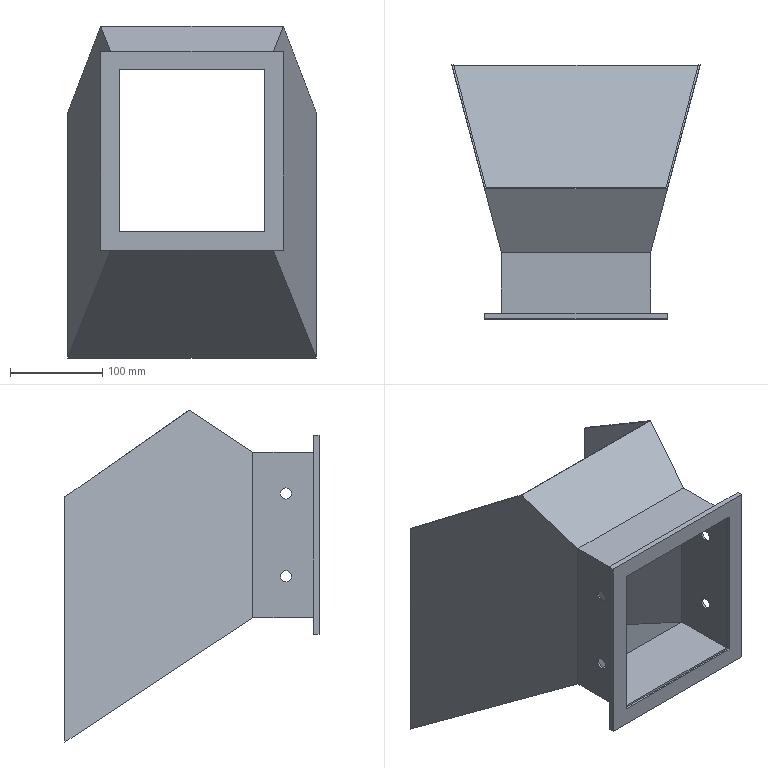Part | NX | 1 solid | 42 faces | box 270 x 276 x 360.692 mm | volume 479442 mm3 | plane 34 | cylinder 8 | commonest cylinder face diameters 12 x8
STEP:
#1=CARTESIAN_POINT('',(51.294,-541.499,2326.086));
#2=VERTEX_POINT('',#1);
#3=CARTESIAN_POINT('',(51.294,-541.499,2314.086));
#4=VERTEX_POINT('',#3);
#5=CARTESIAN_POINT('',(51.294,-541.499,2320.086));
#6=DIRECTION('',(1.,0.,0.));
#7=DIRECTION('',(0.,-1.,0.));
#8=AXIS2_PLACEMENT_3D('',#5,#6,#7);
#9=CIRCLE('',#8,6.);
#10=EDGE_CURVE('',#2,#4,#9,.T.);
#11=ORIENTED_EDGE('',*,*,#10,.T.);
#12=CARTESIAN_POINT('',(49.374,-541.499,2314.086));
#13=VERTEX_POINT('',#12);
#14=CARTESIAN_POINT('',(265.374,-541.499,2314.086));
#15=DIRECTION('',(1.,0.,0.));
#16=VECTOR('',#15,1.);
#17=LINE('',#14,#16);
#18=EDGE_CURVE('',#13,#4,#17,.T.);
#19=ORIENTED_EDGE('',*,*,#18,.F.);
#20=CARTESIAN_POINT('',(49.374,-541.499,2326.086));
#21=VERTEX_POINT('',#20);
#22=CARTESIAN_POINT('',(49.374,-541.499,2320.086));
#23=DIRECTION('',(1.,0.,0.));
#24=DIRECTION('',(0.,-1.,0.));
#25=AXIS2_PLACEMENT_3D('',#22,#23,#24);
#26=CIRCLE('',#25,6.);
#27=EDGE_CURVE('',#21,#13,#26,.T.);
#28=ORIENTED_EDGE('',*,*,#27,.F.);
#29=CARTESIAN_POINT('',(265.374,-541.499,2326.086));
#30=DIRECTION('',(-1.,0.,0.));
#31=VECTOR('',#30,1.);
#32=LINE('',#29,#31);
#33=EDGE_CURVE('',#2,#21,#32,.T.);
#34=ORIENTED_EDGE('',*,*,#33,.F.);
#35=EDGE_LOOP('',(#11,#19,#28,#34));
#36=FACE_OUTER_BOUND('',#35,.T.);
#37=CARTESIAN_POINT('',(265.374,-541.499,2320.086));
#38=DIRECTION('',(-1.,0.,0.));
#39=DIRECTION('',(0.,0.,1.));
#40=AXIS2_PLACEMENT_3D('',#37,#38,#39);
#41=CYLINDRICAL_SURFACE('',#40,6.);
#42=ADVANCED_FACE('',(#36),#41,.F.);
#43=CARTESIAN_POINT('',(211.374,-541.499,2314.086));
#44=VERTEX_POINT('',#43);
#45=CARTESIAN_POINT('',(211.374,-541.499,2326.086));
#46=VERTEX_POINT('',#45);
#47=CARTESIAN_POINT('',(211.374,-541.499,2320.086));
#48=DIRECTION('',(-1.,0.,0.));
#49=DIRECTION('',(0.,1.,0.));
#50=AXIS2_PLACEMENT_3D('',#47,#48,#49);
#51=CIRCLE('',#50,6.);
#52=EDGE_CURVE('',#44,#46,#51,.T.);
#53=ORIENTED_EDGE('',*,*,#52,.F.);
#54=CARTESIAN_POINT('',(209.454,-541.499,2314.086));
#55=VERTEX_POINT('',#54);
#56=CARTESIAN_POINT('',(265.374,-541.499,2314.086));
#57=DIRECTION('',(-1.,0.,0.));
#58=VECTOR('',#57,1.);
#59=LINE('',#56,#58);
#60=EDGE_CURVE('',#44,#55,#59,.T.);
#61=ORIENTED_EDGE('',*,*,#60,.T.);
#62=CARTESIAN_POINT('',(209.454,-541.499,2326.086));
#63=VERTEX_POINT('',#62);
#64=CARTESIAN_POINT('',(209.454,-541.499,2320.086));
#65=DIRECTION('',(-1.,0.,0.));
#66=DIRECTION('',(0.,1.,0.));
#67=AXIS2_PLACEMENT_3D('',#64,#65,#66);
#68=CIRCLE('',#67,6.);
#69=EDGE_CURVE('',#55,#63,#68,.T.);
#70=ORIENTED_EDGE('',*,*,#69,.T.);
#71=CARTESIAN_POINT('',(265.374,-541.499,2326.086));
#72=DIRECTION('',(1.,0.,0.));
#73=VECTOR('',#72,1.);
#74=LINE('',#71,#73);
#75=EDGE_CURVE('',#63,#46,#74,.T.);
#76=ORIENTED_EDGE('',*,*,#75,.T.);
#77=EDGE_LOOP('',(#53,#61,#70,#76));
#78=FACE_OUTER_BOUND('',#77,.T.);
#79=CARTESIAN_POINT('',(265.374,-541.499,2320.086));
#80=DIRECTION('',(-1.,0.,0.));
#81=DIRECTION('',(0.,0.,1.));
#82=AXIS2_PLACEMENT_3D('',#79,#80,#81);
#83=CYLINDRICAL_SURFACE('',#82,6.);
#84=ADVANCED_FACE('',(#78),#83,.F.);
#85=CARTESIAN_POINT('',(51.294,-541.499,2416.086));
#86=VERTEX_POINT('',#85);
#87=CARTESIAN_POINT('',(51.294,-541.499,2404.086));
#88=VERTEX_POINT('',#87);
#89=CARTESIAN_POINT('',(51.294,-541.499,2410.086));
#90=DIRECTION('',(1.,0.,0.));
#91=DIRECTION('',(0.,-1.,0.));
#92=AXIS2_PLACEMENT_3D('',#89,#90,#91);
#93=CIRCLE('',#92,6.);
#94=EDGE_CURVE('',#86,#88,#93,.T.);
#95=ORIENTED_EDGE('',*,*,#94,.T.);
#96=CARTESIAN_POINT('',(49.374,-541.499,2404.086));
#97=VERTEX_POINT('',#96);
#98=CARTESIAN_POINT('',(265.374,-541.499,2404.086));
#99=DIRECTION('',(1.,0.,0.));
#100=VECTOR('',#99,1.);
#101=LINE('',#98,#100);
#102=EDGE_CURVE('',#97,#88,#101,.T.);
#103=ORIENTED_EDGE('',*,*,#102,.F.);
#104=CARTESIAN_POINT('',(49.374,-541.499,2416.086));
#105=VERTEX_POINT('',#104);
#106=CARTESIAN_POINT('',(49.374,-541.499,2410.086));
#107=DIRECTION('',(1.,0.,0.));
#108=DIRECTION('',(0.,-1.,0.));
#109=AXIS2_PLACEMENT_3D('',#106,#107,#108);
#110=CIRCLE('',#109,6.);
#111=EDGE_CURVE('',#105,#97,#110,.T.);
#112=ORIENTED_EDGE('',*,*,#111,.F.);
#113=CARTESIAN_POINT('',(265.374,-541.499,2416.086));
#114=DIRECTION('',(-1.,0.,0.));
#115=VECTOR('',#114,1.);
#116=LINE('',#113,#115);
#117=EDGE_CURVE('',#86,#105,#116,.T.);
#118=ORIENTED_EDGE('',*,*,#117,.F.);
#119=EDGE_LOOP('',(#95,#103,#112,#118));
#120=FACE_OUTER_BOUND('',#119,.T.);
#121=CARTESIAN_POINT('',(265.374,-541.499,2410.086));
#122=DIRECTION('',(-1.,0.,0.));
#123=DIRECTION('',(0.,0.,1.));
#124=AXIS2_PLACEMENT_3D('',#121,#122,#123);
#125=CYLINDRICAL_SURFACE('',#124,6.);
#126=ADVANCED_FACE('',(#120),#125,.F.);
#127=CARTESIAN_POINT('',(211.374,-541.499,2404.086));
#128=VERTEX_POINT('',#127);
#129=CARTESIAN_POINT('',(211.374,-541.499,2416.086));
#130=VERTEX_POINT('',#129);
#131=CARTESIAN_POINT('',(211.374,-541.499,2410.086));
#132=DIRECTION('',(-1.,0.,0.));
#133=DIRECTION('',(0.,1.,0.));
#134=AXIS2_PLACEMENT_3D('',#131,#132,#133);
#135=CIRCLE('',#134,6.);
#136=EDGE_CURVE('',#128,#130,#135,.T.);
#137=ORIENTED_EDGE('',*,*,#136,.F.);
#138=CARTESIAN_POINT('',(209.454,-541.499,2404.086));
#139=VERTEX_POINT('',#138);
#140=CARTESIAN_POINT('',(265.374,-541.499,2404.086));
#141=DIRECTION('',(1.,0.,0.));
#142=VECTOR('',#141,1.);
#143=LINE('',#140,#142);
#144=EDGE_CURVE('',#139,#128,#143,.T.);
#145=ORIENTED_EDGE('',*,*,#144,.F.);
#146=CARTESIAN_POINT('',(209.454,-541.499,2416.086));
#147=VERTEX_POINT('',#146);
#148=CARTESIAN_POINT('',(209.454,-541.499,2410.086));
#149=DIRECTION('',(-1.,0.,0.));
#150=DIRECTION('',(0.,1.,0.));
#151=AXIS2_PLACEMENT_3D('',#148,#149,#150);
#152=CIRCLE('',#151,6.);
#153=EDGE_CURVE('',#139,#147,#152,.T.);
#154=ORIENTED_EDGE('',*,*,#153,.T.);
#155=CARTESIAN_POINT('',(265.374,-541.499,2416.086));
#156=DIRECTION('',(-1.,0.,0.));
#157=VECTOR('',#156,1.);
#158=LINE('',#155,#157);
#159=EDGE_CURVE('',#130,#147,#158,.T.);
#160=ORIENTED_EDGE('',*,*,#159,.F.);
#161=EDGE_LOOP('',(#137,#145,#154,#160));
#162=FACE_OUTER_BOUND('',#161,.T.);
#163=CARTESIAN_POINT('',(265.374,-541.499,2410.086));
#164=DIRECTION('',(-1.,0.,0.));
#165=DIRECTION('',(0.,0.,1.));
#166=AXIS2_PLACEMENT_3D('',#163,#164,#165);
#167=CYLINDRICAL_SURFACE('',#166,6.);
#168=ADVANCED_FACE('',(#162),#167,.F.);
#169=CARTESIAN_POINT('',(-4.626,-301.499,2140.086));
#170=VERTEX_POINT('',#169);
#171=CARTESIAN_POINT('',(-4.626,-301.499,2406.357));
#172=VERTEX_POINT('',#171);
#173=CARTESIAN_POINT('',(-4.626,-301.499,2590.086));
#174=DIRECTION('',(0.,0.,1.));
#175=VECTOR('',#174,1.);
#176=LINE('',#173,#175);
#177=EDGE_CURVE('',#170,#172,#176,.T.);
#178=ORIENTED_EDGE('',*,*,#177,.T.);
#179=CARTESIAN_POINT('',(-2.64,-301.499,2406.357));
#180=VERTEX_POINT('',#179);
#181=CARTESIAN_POINT('',(265.374,-301.499,2406.357));
#182=DIRECTION('',(1.,0.,0.));
#183=VECTOR('',#182,1.);
#184=LINE('',#181,#183);
#185=EDGE_CURVE('',#172,#180,#184,.T.);
#186=ORIENTED_EDGE('',*,*,#185,.T.);
#187=CARTESIAN_POINT('',(-2.64,-301.499,2142.389));
#188=VERTEX_POINT('',#187);
#189=CARTESIAN_POINT('',(-2.64,-301.499,2590.086));
#190=DIRECTION('',(0.,0.,1.));
#191=VECTOR('',#190,1.);
#192=LINE('',#189,#191);
#193=EDGE_CURVE('',#188,#180,#192,.T.);
#194=ORIENTED_EDGE('',*,*,#193,.F.);
#195=CARTESIAN_POINT('',(263.387,-301.499,2142.389));
#196=VERTEX_POINT('',#195);
#197=CARTESIAN_POINT('',(265.374,-301.499,2142.389));
#198=DIRECTION('',(-1.,0.,0.));
#199=VECTOR('',#198,1.);
#200=LINE('',#197,#199);
#201=EDGE_CURVE('',#196,#188,#200,.T.);
#202=ORIENTED_EDGE('',*,*,#201,.F.);
#203=CARTESIAN_POINT('',(263.387,-301.499,2406.357));
#204=VERTEX_POINT('',#203);
#205=CARTESIAN_POINT('',(263.387,-301.499,2140.086));
#206=DIRECTION('',(0.,0.,1.));
#207=VECTOR('',#206,1.);
#208=LINE('',#205,#207);
#209=EDGE_CURVE('',#196,#204,#208,.T.);
#210=ORIENTED_EDGE('',*,*,#209,.T.);
#211=CARTESIAN_POINT('',(265.374,-301.499,2406.357));
#212=VERTEX_POINT('',#211);
#213=CARTESIAN_POINT('',(265.374,-301.499,2406.357));
#214=DIRECTION('',(1.,0.,0.));
#215=VECTOR('',#214,1.);
#216=LINE('',#213,#215);
#217=EDGE_CURVE('',#204,#212,#216,.T.);
#218=ORIENTED_EDGE('',*,*,#217,.T.);
#219=CARTESIAN_POINT('',(265.374,-301.499,2140.086));
#220=VERTEX_POINT('',#219);
#221=CARTESIAN_POINT('',(265.374,-301.499,2590.086));
#222=DIRECTION('',(0.,0.,1.));
#223=VECTOR('',#222,1.);
#224=LINE('',#221,#223);
#225=EDGE_CURVE('',#220,#212,#224,.T.);
#226=ORIENTED_EDGE('',*,*,#225,.F.);
#227=CARTESIAN_POINT('',(265.374,-301.499,2140.086));
#228=DIRECTION('',(-1.,0.,0.));
#229=VECTOR('',#228,1.);
#230=LINE('',#227,#229);
#231=EDGE_CURVE('',#220,#170,#230,.T.);
#232=ORIENTED_EDGE('',*,*,#231,.T.);
#233=EDGE_LOOP('',(#178,#186,#194,#202,#210,#218,#226,#232));
#234=FACE_OUTER_BOUND('',#233,.T.);
#235=CARTESIAN_POINT('',(265.374,-301.499,2590.086));
#236=DIRECTION('',(0.,-1.,0.));
#237=DIRECTION('',(0.,0.,-1.));
#238=AXIS2_PLACEMENT_3D('',#235,#236,#237);
#239=PLANE('',#238);
#240=ADVANCED_FACE('',(#234),#239,.F.);
#241=CARTESIAN_POINT('',(211.374,-571.499,2455.086));
#242=VERTEX_POINT('',#241);
#243=CARTESIAN_POINT('',(49.374,-571.499,2455.086));
#244=VERTEX_POINT('',#243);
#245=CARTESIAN_POINT('',(265.374,-571.499,2455.086));
#246=DIRECTION('',(-1.,0.,0.));
#247=VECTOR('',#246,1.);
#248=LINE('',#245,#247);
#249=EDGE_CURVE('',#242,#244,#248,.T.);
#250=ORIENTED_EDGE('',*,*,#249,.F.);
#251=CARTESIAN_POINT('',(211.374,-505.499,2455.086));
#252=VERTEX_POINT('',#251);
#253=CARTESIAN_POINT('',(211.374,-571.499,2455.086));
#254=DIRECTION('',(0.,1.,0.));
#255=VECTOR('',#254,1.);
#256=LINE('',#253,#255);
#257=EDGE_CURVE('',#242,#252,#256,.T.);
#258=ORIENTED_EDGE('',*,*,#257,.T.);
#259=CARTESIAN_POINT('',(49.374,-505.499,2455.086));
#260=VERTEX_POINT('',#259);
#261=CARTESIAN_POINT('',(265.374,-505.499,2455.086));
#262=DIRECTION('',(-1.,0.,0.));
#263=VECTOR('',#262,1.);
#264=LINE('',#261,#263);
#265=EDGE_CURVE('',#252,#260,#264,.T.);
#266=ORIENTED_EDGE('',*,*,#265,.T.);
#267=CARTESIAN_POINT('',(49.374,-571.499,2455.086));
#268=DIRECTION('',(0.,-1.,0.));
#269=VECTOR('',#268,1.);
#270=LINE('',#267,#269);
#271=EDGE_CURVE('',#260,#244,#270,.T.);
#272=ORIENTED_EDGE('',*,*,#271,.T.);
#273=EDGE_LOOP('',(#250,#258,#266,#272));
#274=FACE_OUTER_BOUND('',#273,.T.);
#275=CARTESIAN_POINT('',(265.374,-571.499,2455.086));
#276=DIRECTION('',(0.,0.,-1.));
#277=DIRECTION('',(-1.,0.,0.));
#278=AXIS2_PLACEMENT_3D('',#275,#276,#277);
#279=PLANE('',#278);
#280=ADVANCED_FACE('',(#274),#279,.F.);
#281=CARTESIAN_POINT('',(211.374,-505.499,2275.086));
#282=VERTEX_POINT('',#281);
#283=CARTESIAN_POINT('',(49.374,-505.499,2275.086));
#284=VERTEX_POINT('',#283);
#285=CARTESIAN_POINT('',(265.374,-505.499,2275.086));
#286=DIRECTION('',(-1.,0.,0.));
#287=VECTOR('',#286,1.);
#288=LINE('',#285,#287);
#289=EDGE_CURVE('',#282,#284,#288,.T.);
#290=ORIENTED_EDGE('',*,*,#289,.F.);
#291=CARTESIAN_POINT('',(211.374,-571.499,2275.086));
#292=VERTEX_POINT('',#291);
#293=CARTESIAN_POINT('',(211.374,-571.499,2275.086));
#294=DIRECTION('',(0.,-1.,0.));
#295=VECTOR('',#294,1.);
#296=LINE('',#293,#295);
#297=EDGE_CURVE('',#282,#292,#296,.T.);
#298=ORIENTED_EDGE('',*,*,#297,.T.);
#299=CARTESIAN_POINT('',(49.374,-571.499,2275.086));
#300=VERTEX_POINT('',#299);
#301=CARTESIAN_POINT('',(265.374,-571.499,2275.086));
#302=DIRECTION('',(-1.,0.,0.));
#303=VECTOR('',#302,1.);
#304=LINE('',#301,#303);
#305=EDGE_CURVE('',#292,#300,#304,.T.);
#306=ORIENTED_EDGE('',*,*,#305,.T.);
#307=CARTESIAN_POINT('',(49.374,-571.499,2275.086));
#308=DIRECTION('',(0.,1.,0.));
#309=VECTOR('',#308,1.);
#310=LINE('',#307,#309);
#311=EDGE_CURVE('',#300,#284,#310,.T.);
#312=ORIENTED_EDGE('',*,*,#311,.T.);
#313=EDGE_LOOP('',(#290,#298,#306,#312));
#314=FACE_OUTER_BOUND('',#313,.T.);
#315=CARTESIAN_POINT('',(265.374,-571.499,2275.086));
#316=DIRECTION('',(0.,0.,1.));
#317=DIRECTION('',(0.,-1.,0.));
#318=AXIS2_PLACEMENT_3D('',#315,#316,#317);
#319=PLANE('',#318);
#320=ADVANCED_FACE('',(#314),#319,.F.);
#321=ORIENTED_EDGE('',*,*,#231,.F.);
#322=CARTESIAN_POINT('',(265.374,-301.499,2140.086));
#323=DIRECTION('',(-0.2156,-0.8143,0.5389));
#324=VECTOR('',#323,1.);
#325=LINE('',#322,#324);
#326=EDGE_CURVE('',#220,#282,#325,.T.);
#327=ORIENTED_EDGE('',*,*,#326,.T.);
#328=ORIENTED_EDGE('',*,*,#289,.T.);
#329=CARTESIAN_POINT('',(7.919,-348.894,2171.45));
#330=DIRECTION('',(-0.2156,0.8143,-0.5389));
#331=VECTOR('',#330,1.);
#332=LINE('',#329,#331);
#333=EDGE_CURVE('',#284,#170,#332,.T.);
#334=ORIENTED_EDGE('',*,*,#333,.T.);
#335=EDGE_LOOP('',(#321,#327,#328,#334));
#336=FACE_OUTER_BOUND('',#335,.T.);
#337=CARTESIAN_POINT('',(265.374,-301.499,2140.086));
#338=DIRECTION('',(0.,0.5519,0.8339));
#339=DIRECTION('',(0.,-0.8339,0.5519));
#340=AXIS2_PLACEMENT_3D('',#337,#338,#339);
#341=PLANE('',#340);
#342=ADVANCED_FACE('',(#336),#341,.F.);
#343=CARTESIAN_POINT('',(229.65,-436.453,2500.778));
#344=VERTEX_POINT('',#343);
#345=CARTESIAN_POINT('',(265.374,-301.499,2590.086));
#346=DIRECTION('',(0.2156,0.8143,0.5389));
#347=VECTOR('',#346,1.);
#348=LINE('',#345,#347);
#349=EDGE_CURVE('',#252,#344,#348,.T.);
#350=ORIENTED_EDGE('',*,*,#349,.T.);
#351=CARTESIAN_POINT('',(31.097,-436.453,2500.778));
#352=VERTEX_POINT('',#351);
#353=CARTESIAN_POINT('',(265.374,-436.453,2500.778));
#354=DIRECTION('',(-1.,0.,0.));
#355=VECTOR('',#354,1.);
#356=LINE('',#353,#355);
#357=EDGE_CURVE('',#344,#352,#356,.T.);
#358=ORIENTED_EDGE('',*,*,#357,.T.);
#359=CARTESIAN_POINT('',(7.919,-348.894,2558.722));
#360=DIRECTION('',(0.2156,-0.8143,-0.5389));
#361=VECTOR('',#360,1.);
#362=LINE('',#359,#361);
#363=EDGE_CURVE('',#352,#260,#362,.T.);
#364=ORIENTED_EDGE('',*,*,#363,.T.);
#365=ORIENTED_EDGE('',*,*,#265,.F.);
#366=EDGE_LOOP('',(#350,#358,#364,#365));
#367=FACE_OUTER_BOUND('',#366,.T.);
#368=CARTESIAN_POINT('',(265.374,-301.499,2590.086));
#369=DIRECTION('',(0.,0.5519,-0.8339));
#370=DIRECTION('',(0.,0.8339,0.5519));
#371=AXIS2_PLACEMENT_3D('',#368,#369,#370);
#372=PLANE('',#371);
#373=ADVANCED_FACE('',(#367),#372,.F.);
#374=ORIENTED_EDGE('',*,*,#27,.T.);
#375=CARTESIAN_POINT('',(49.374,-541.499,2320.086));
#376=DIRECTION('',(1.,0.,0.));
#377=DIRECTION('',(0.,-1.,0.));
#378=AXIS2_PLACEMENT_3D('',#375,#376,#377);
#379=CIRCLE('',#378,6.);
#380=EDGE_CURVE('',#13,#21,#379,.T.);
#381=ORIENTED_EDGE('',*,*,#380,.T.);
#382=EDGE_LOOP('',(#374,#381));
#383=FACE_BOUND('',#382,.T.);
#384=ORIENTED_EDGE('',*,*,#111,.T.);
#385=CARTESIAN_POINT('',(49.374,-541.499,2410.086));
#386=DIRECTION('',(1.,0.,0.));
#387=DIRECTION('',(0.,-1.,0.));
#388=AXIS2_PLACEMENT_3D('',#385,#386,#387);
#389=CIRCLE('',#388,6.);
#390=EDGE_CURVE('',#97,#105,#389,.T.);
#391=ORIENTED_EDGE('',*,*,#390,.T.);
#392=EDGE_LOOP('',(#384,#391));
#393=FACE_BOUND('',#392,.T.);
#394=CARTESIAN_POINT('',(49.374,-505.499,2140.086));
#395=DIRECTION('',(0.,0.,1.));
#396=VECTOR('',#395,1.);
#397=LINE('',#394,#396);
#398=EDGE_CURVE('',#284,#260,#397,.T.);
#399=ORIENTED_EDGE('',*,*,#398,.F.);
#400=ORIENTED_EDGE('',*,*,#311,.F.);
#401=CARTESIAN_POINT('',(49.374,-571.499,2140.086));
#402=DIRECTION('',(0.,0.,1.));
#403=VECTOR('',#402,1.);
#404=LINE('',#401,#403);
#405=EDGE_CURVE('',#300,#244,#404,.T.);
#406=ORIENTED_EDGE('',*,*,#405,.T.);
#407=ORIENTED_EDGE('',*,*,#271,.F.);
#408=EDGE_LOOP('',(#399,#400,#406,#407));
#409=FACE_BOUND('',#408,.T.);
#410=CARTESIAN_POINT('',(49.374,-505.499,2140.086));
#411=DIRECTION('',(1.,0.,0.));
#412=DIRECTION('',(0.,-1.,0.));
#413=AXIS2_PLACEMENT_3D('',#410,#411,#412);
#414=PLANE('',#413);
#415=ADVANCED_FACE('',(#383,#393,#409),#414,.F.);
#416=ORIENTED_EDGE('',*,*,#363,.F.);
#417=CARTESIAN_POINT('',(-36.246,-182.046,2322.78));
#418=DIRECTION('',(-0.212,0.8007,-0.5602));
#419=VECTOR('',#418,1.);
#420=LINE('',#417,#419);
#421=EDGE_CURVE('',#352,#172,#420,.T.);
#422=ORIENTED_EDGE('',*,*,#421,.T.);
#423=ORIENTED_EDGE('',*,*,#177,.F.);
#424=ORIENTED_EDGE('',*,*,#333,.F.);
#425=ORIENTED_EDGE('',*,*,#398,.T.);
#426=EDGE_LOOP('',(#416,#422,#423,#424,#425));
#427=FACE_OUTER_BOUND('',#426,.T.);
#428=CARTESIAN_POINT('',(-4.626,-301.499,2140.086));
#429=DIRECTION('',(0.9667,0.2559,0.));
#430=DIRECTION('',(0.2559,-0.9667,0.));
#431=AXIS2_PLACEMENT_3D('',#428,#429,#430);
#432=PLANE('',#431);
#433=ADVANCED_FACE('',(#427),#432,.F.);
#434=CARTESIAN_POINT('',(211.374,-541.499,2320.086));
#435=DIRECTION('',(-1.,0.,0.));
#436=DIRECTION('',(0.,1.,0.));
#437=AXIS2_PLACEMENT_3D('',#434,#435,#436);
#438=CIRCLE('',#437,6.);
#439=EDGE_CURVE('',#46,#44,#438,.T.);
#440=ORIENTED_EDGE('',*,*,#439,.T.);
#441=ORIENTED_EDGE('',*,*,#52,.T.);
#442=EDGE_LOOP('',(#440,#441));
#443=FACE_BOUND('',#442,.T.);
#444=CARTESIAN_POINT('',(211.374,-541.499,2410.086));
#445=DIRECTION('',(-1.,0.,0.));
#446=DIRECTION('',(0.,1.,0.));
#447=AXIS2_PLACEMENT_3D('',#444,#445,#446);
#448=CIRCLE('',#447,6.);
#449=EDGE_CURVE('',#130,#128,#448,.T.);
#450=ORIENTED_EDGE('',*,*,#449,.T.);
#451=ORIENTED_EDGE('',*,*,#136,.T.);
#452=EDGE_LOOP('',(#450,#451));
#453=FACE_BOUND('',#452,.T.);
#454=CARTESIAN_POINT('',(211.374,-571.499,2140.086));
#455=DIRECTION('',(0.,0.,1.));
#456=VECTOR('',#455,1.);
#457=LINE('',#454,#456);
#458=EDGE_CURVE('',#292,#242,#457,.T.);
#459=ORIENTED_EDGE('',*,*,#458,.F.);
#460=ORIENTED_EDGE('',*,*,#297,.F.);
#461=CARTESIAN_POINT('',(211.374,-505.499,2140.086));
#462=DIRECTION('',(0.,0.,1.));
#463=VECTOR('',#462,1.);
#464=LINE('',#461,#463);
#465=EDGE_CURVE('',#282,#252,#464,.T.);
#466=ORIENTED_EDGE('',*,*,#465,.T.);
#467=ORIENTED_EDGE('',*,*,#257,.F.);
#468=EDGE_LOOP('',(#459,#460,#466,#467));
#469=FACE_BOUND('',#468,.T.);
#470=CARTESIAN_POINT('',(211.374,-505.499,2140.086));
#471=DIRECTION('',(-1.,0.,0.));
#472=DIRECTION('',(0.,1.,0.));
#473=AXIS2_PLACEMENT_3D('',#470,#471,#472);
#474=PLANE('',#473);
#475=ADVANCED_FACE('',(#443,#453,#469),#474,.F.);
#476=ORIENTED_EDGE('',*,*,#225,.T.);
#477=CARTESIAN_POINT('',(296.994,-182.046,2322.78));
#478=DIRECTION('',(-0.212,-0.8007,0.5602));
#479=VECTOR('',#478,1.);
#480=LINE('',#477,#479);
#481=EDGE_CURVE('',#212,#344,#480,.T.);
#482=ORIENTED_EDGE('',*,*,#481,.T.);
#483=ORIENTED_EDGE('',*,*,#349,.F.);
#484=ORIENTED_EDGE('',*,*,#465,.F.);
#485=ORIENTED_EDGE('',*,*,#326,.F.);
#486=EDGE_LOOP('',(#476,#482,#483,#484,#485));
#487=FACE_OUTER_BOUND('',#486,.T.);
#488=CARTESIAN_POINT('',(265.374,-301.499,2140.086));
#489=DIRECTION('',(-0.9667,0.2559,0.));
#490=DIRECTION('',(0.2559,0.9667,0.));
#491=AXIS2_PLACEMENT_3D('',#488,#489,#490);
#492=PLANE('',#491);
#493=ADVANCED_FACE('',(#487),#492,.F.);
#494=CARTESIAN_POINT('',(229.374,-571.499,2473.086));
#495=VERTEX_POINT('',#494);
#496=CARTESIAN_POINT('',(31.374,-571.499,2473.086));
#497=VERTEX_POINT('',#496);
#498=CARTESIAN_POINT('',(229.374,-571.499,2473.086));
#499=DIRECTION('',(-1.,0.,0.));
#500=VECTOR('',#499,1.);
#501=LINE('',#498,#500);
#502=EDGE_CURVE('',#495,#497,#501,.T.);
#503=ORIENTED_EDGE('',*,*,#502,.F.);
#504=CARTESIAN_POINT('',(229.374,-571.499,2257.086));
#505=VERTEX_POINT('',#504);
#506=CARTESIAN_POINT('',(229.374,-571.499,2257.086));
#507=DIRECTION('',(0.,0.,1.));
#508=VECTOR('',#507,1.);
#509=LINE('',#506,#508);
#510=EDGE_CURVE('',#505,#495,#509,.T.);
#511=ORIENTED_EDGE('',*,*,#510,.F.);
#512=CARTESIAN_POINT('',(31.374,-571.499,2257.086));
#513=VERTEX_POINT('',#512);
#514=CARTESIAN_POINT('',(31.374,-571.499,2257.086));
#515=DIRECTION('',(1.,0.,0.));
#516=VECTOR('',#515,1.);
#517=LINE('',#514,#516);
#518=EDGE_CURVE('',#513,#505,#517,.T.);
#519=ORIENTED_EDGE('',*,*,#518,.F.);
#520=CARTESIAN_POINT('',(31.374,-571.499,2473.086));
#521=DIRECTION('',(0.,0.,-1.));
#522=VECTOR('',#521,1.);
#523=LINE('',#520,#522);
#524=EDGE_CURVE('',#497,#513,#523,.T.);
#525=ORIENTED_EDGE('',*,*,#524,.F.);
#526=EDGE_LOOP('',(#503,#511,#519,#525));
#527=FACE_BOUND('',#526,.T.);
#528=ORIENTED_EDGE('',*,*,#249,.T.);
#529=ORIENTED_EDGE('',*,*,#405,.F.);
#530=ORIENTED_EDGE('',*,*,#305,.F.);
#531=ORIENTED_EDGE('',*,*,#458,.T.);
#532=EDGE_LOOP('',(#528,#529,#530,#531));
#533=FACE_BOUND('',#532,.T.);
#534=CARTESIAN_POINT('',(31.374,-571.499,2473.086));
#535=DIRECTION('',(0.,-1.,0.));
#536=DIRECTION('',(-1.,0.,0.));
#537=AXIS2_PLACEMENT_3D('',#534,#535,#536);
#538=PLANE('',#537);
#539=ADVANCED_FACE('',(#527,#533),#538,.F.);
#540=ORIENTED_EDGE('',*,*,#502,.T.);
#541=CARTESIAN_POINT('',(31.374,-577.499,2473.086));
#542=VERTEX_POINT('',#541);
#543=CARTESIAN_POINT('',(31.374,-577.499,2473.086));
#544=DIRECTION('',(0.,1.,0.));
#545=VECTOR('',#544,1.);
#546=LINE('',#543,#545);
#547=EDGE_CURVE('',#542,#497,#546,.T.);
#548=ORIENTED_EDGE('',*,*,#547,.F.);
#549=CARTESIAN_POINT('',(229.374,-577.499,2473.086));
#550=VERTEX_POINT('',#549);
#551=CARTESIAN_POINT('',(229.374,-577.499,2473.086));
#552=DIRECTION('',(-1.,0.,0.));
#553=VECTOR('',#552,1.);
#554=LINE('',#551,#553);
#555=EDGE_CURVE('',#550,#542,#554,.T.);
#556=ORIENTED_EDGE('',*,*,#555,.F.);
#557=CARTESIAN_POINT('',(229.374,-577.499,2473.086));
#558=DIRECTION('',(0.,1.,0.));
#559=VECTOR('',#558,1.);
#560=LINE('',#557,#559);
#561=EDGE_CURVE('',#550,#495,#560,.T.);
#562=ORIENTED_EDGE('',*,*,#561,.T.);
#563=EDGE_LOOP('',(#540,#548,#556,#562));
#564=FACE_OUTER_BOUND('',#563,.T.);
#565=CARTESIAN_POINT('',(229.374,-577.499,2473.086));
#566=DIRECTION('',(0.,0.,-1.));
#567=DIRECTION('',(-1.,0.,0.));
#568=AXIS2_PLACEMENT_3D('',#565,#566,#567);
#569=PLANE('',#568);
#570=ADVANCED_FACE('',(#564),#569,.F.);
#571=ORIENTED_EDGE('',*,*,#524,.T.);
#572=CARTESIAN_POINT('',(31.374,-577.499,2257.086));
#573=VERTEX_POINT('',#572);
#574=CARTESIAN_POINT('',(31.374,-577.499,2257.086));
#575=DIRECTION('',(0.,1.,0.));
#576=VECTOR('',#575,1.);
#577=LINE('',#574,#576);
#578=EDGE_CURVE('',#573,#513,#577,.T.);
#579=ORIENTED_EDGE('',*,*,#578,.F.);
#580=CARTESIAN_POINT('',(31.374,-577.499,2473.086));
#581=DIRECTION('',(0.,0.,-1.));
#582=VECTOR('',#581,1.);
#583=LINE('',#580,#582);
#584=EDGE_CURVE('',#542,#573,#583,.T.);
#585=ORIENTED_EDGE('',*,*,#584,.F.);
#586=ORIENTED_EDGE('',*,*,#547,.T.);
#587=EDGE_LOOP('',(#571,#579,#585,#586));
#588=FACE_OUTER_BOUND('',#587,.T.);
#589=CARTESIAN_POINT('',(31.374,-577.499,2473.086));
#590=DIRECTION('',(1.,0.,0.));
#591=DIRECTION('',(0.,0.,-1.));
#592=AXIS2_PLACEMENT_3D('',#589,#590,#591);
#593=PLANE('',#592);
#594=ADVANCED_FACE('',(#588),#593,.F.);
#595=ORIENTED_EDGE('',*,*,#518,.T.);
#596=CARTESIAN_POINT('',(229.374,-577.499,2257.086));
#597=VERTEX_POINT('',#596);
#598=CARTESIAN_POINT('',(229.374,-577.499,2257.086));
#599=DIRECTION('',(0.,1.,0.));
#600=VECTOR('',#599,1.);
#601=LINE('',#598,#600);
#602=EDGE_CURVE('',#597,#505,#601,.T.);
#603=ORIENTED_EDGE('',*,*,#602,.F.);
#604=CARTESIAN_POINT('',(31.374,-577.499,2257.086));
#605=DIRECTION('',(1.,0.,0.));
#606=VECTOR('',#605,1.);
#607=LINE('',#604,#606);
#608=EDGE_CURVE('',#573,#597,#607,.T.);
#609=ORIENTED_EDGE('',*,*,#608,.F.);
#610=ORIENTED_EDGE('',*,*,#578,.T.);
#611=EDGE_LOOP('',(#595,#603,#609,#610));
#612=FACE_OUTER_BOUND('',#611,.T.);
#613=CARTESIAN_POINT('',(31.374,-577.499,2257.086));
#614=DIRECTION('',(0.,0.,1.));
#615=DIRECTION('',(1.,0.,0.));
#616=AXIS2_PLACEMENT_3D('',#613,#614,#615);
#617=PLANE('',#616);
#618=ADVANCED_FACE('',(#612),#617,.F.);
#619=ORIENTED_EDGE('',*,*,#510,.T.);
#620=ORIENTED_EDGE('',*,*,#561,.F.);
#621=CARTESIAN_POINT('',(229.374,-577.499,2257.086));
#622=DIRECTION('',(0.,0.,1.));
#623=VECTOR('',#622,1.);
#624=LINE('',#621,#623);
#625=EDGE_CURVE('',#597,#550,#624,.T.);
#626=ORIENTED_EDGE('',*,*,#625,.F.);
#627=ORIENTED_EDGE('',*,*,#602,.T.);
#628=EDGE_LOOP('',(#619,#620,#626,#627));
#629=FACE_OUTER_BOUND('',#628,.T.);
#630=CARTESIAN_POINT('',(229.374,-577.499,2257.086));
#631=DIRECTION('',(-1.,0.,0.));
#632=DIRECTION('',(0.,0.,1.));
#633=AXIS2_PLACEMENT_3D('',#630,#631,#632);
#634=PLANE('',#633);
#635=ADVANCED_FACE('',(#629),#634,.F.);
#636=CARTESIAN_POINT('',(209.454,-577.499,2453.166));
#637=VERTEX_POINT('',#636);
#638=CARTESIAN_POINT('',(51.294,-577.499,2453.166));
#639=VERTEX_POINT('',#638);
#640=CARTESIAN_POINT('',(209.454,-577.499,2453.166));
#641=DIRECTION('',(-1.,0.,0.));
#642=VECTOR('',#641,1.);
#643=LINE('',#640,#642);
#644=EDGE_CURVE('',#637,#639,#643,.T.);
#645=ORIENTED_EDGE('',*,*,#644,.F.);
#646=CARTESIAN_POINT('',(209.454,-577.499,2277.006));
#647=VERTEX_POINT('',#646);
#648=CARTESIAN_POINT('',(209.454,-577.499,2453.166));
#649=DIRECTION('',(0.,0.,1.));
#650=VECTOR('',#649,1.);
#651=LINE('',#648,#650);
#652=EDGE_CURVE('',#647,#637,#651,.T.);
#653=ORIENTED_EDGE('',*,*,#652,.F.);
#654=CARTESIAN_POINT('',(51.294,-577.499,2277.006));
#655=VERTEX_POINT('',#654);
#656=CARTESIAN_POINT('',(209.454,-577.499,2277.006));
#657=DIRECTION('',(1.,0.,0.));
#658=VECTOR('',#657,1.);
#659=LINE('',#656,#658);
#660=EDGE_CURVE('',#655,#647,#659,.T.);
#661=ORIENTED_EDGE('',*,*,#660,.F.);
#662=CARTESIAN_POINT('',(51.294,-577.499,2453.166));
#663=DIRECTION('',(0.,0.,-1.));
#664=VECTOR('',#663,1.);
#665=LINE('',#662,#664);
#666=EDGE_CURVE('',#639,#655,#665,.T.);
#667=ORIENTED_EDGE('',*,*,#666,.F.);
#668=EDGE_LOOP('',(#645,#653,#661,#667));
#669=FACE_BOUND('',#668,.T.);
#670=ORIENTED_EDGE('',*,*,#555,.T.);
#671=ORIENTED_EDGE('',*,*,#584,.T.);
#672=ORIENTED_EDGE('',*,*,#608,.T.);
#673=ORIENTED_EDGE('',*,*,#625,.T.);
#674=EDGE_LOOP('',(#670,#671,#672,#673));
#675=FACE_BOUND('',#674,.T.);
#676=CARTESIAN_POINT('',(31.374,-577.499,2473.086));
#677=DIRECTION('',(0.,-1.,0.));
#678=DIRECTION('',(-1.,0.,0.));
#679=AXIS2_PLACEMENT_3D('',#676,#677,#678);
#680=PLANE('',#679);
#681=ADVANCED_FACE('',(#669,#675),#680,.T.);
#682=CARTESIAN_POINT('',(209.454,-573.419,2453.166));
#683=VERTEX_POINT('',#682);
#684=CARTESIAN_POINT('',(51.294,-573.419,2453.166));
#685=VERTEX_POINT('',#684);
#686=CARTESIAN_POINT('',(265.374,-573.419,2453.166));
#687=DIRECTION('',(-1.,0.,0.));
#688=VECTOR('',#687,1.);
#689=LINE('',#686,#688);
#690=EDGE_CURVE('',#683,#685,#689,.T.);
#691=ORIENTED_EDGE('',*,*,#690,.T.);
#692=CARTESIAN_POINT('',(51.294,-505.249,2453.166));
#693=VERTEX_POINT('',#692);
#694=CARTESIAN_POINT('',(51.294,-571.499,2453.166));
#695=DIRECTION('',(0.,-1.,0.));
#696=VECTOR('',#695,1.);
#697=LINE('',#694,#696);
#698=EDGE_CURVE('',#693,#685,#697,.T.);
#699=ORIENTED_EDGE('',*,*,#698,.F.);
#700=CARTESIAN_POINT('',(51.207,-504.922,2453.166));
#701=VERTEX_POINT('',#700);
#702=CARTESIAN_POINT('',(81.7,-620.119,2453.166));
#703=DIRECTION('',(0.2559,-0.9667,0.));
#704=VECTOR('',#703,1.);
#705=LINE('',#702,#704);
#706=EDGE_CURVE('',#701,#693,#705,.T.);
#707=ORIENTED_EDGE('',*,*,#706,.F.);
#708=CARTESIAN_POINT('',(209.54,-504.922,2453.166));
#709=VERTEX_POINT('',#708);
#710=CARTESIAN_POINT('',(265.374,-504.922,2453.166));
#711=DIRECTION('',(-1.,0.,0.));
#712=VECTOR('',#711,1.);
#713=LINE('',#710,#712);
#714=EDGE_CURVE('',#709,#701,#713,.T.);
#715=ORIENTED_EDGE('',*,*,#714,.F.);
#716=CARTESIAN_POINT('',(209.454,-505.249,2453.166));
#717=VERTEX_POINT('',#716);
#718=CARTESIAN_POINT('',(196.727,-553.328,2453.166));
#719=DIRECTION('',(0.2559,0.9667,0.));
#720=VECTOR('',#719,1.);
#721=LINE('',#718,#720);
#722=EDGE_CURVE('',#717,#709,#721,.T.);
#723=ORIENTED_EDGE('',*,*,#722,.F.);
#724=CARTESIAN_POINT('',(209.454,-571.499,2453.166));
#725=DIRECTION('',(0.,1.,0.));
#726=VECTOR('',#725,1.);
#727=LINE('',#724,#726);
#728=EDGE_CURVE('',#683,#717,#727,.T.);
#729=ORIENTED_EDGE('',*,*,#728,.F.);
#730=EDGE_LOOP('',(#691,#699,#707,#715,#723,#729));
#731=FACE_OUTER_BOUND('',#730,.T.);
#732=CARTESIAN_POINT('',(265.374,-571.499,2453.166));
#733=DIRECTION('',(0.,0.,-1.));
#734=DIRECTION('',(-1.,0.,0.));
#735=AXIS2_PLACEMENT_3D('',#732,#733,#734);
#736=PLANE('',#735);
#737=ADVANCED_FACE('',(#731),#736,.T.);
#738=CARTESIAN_POINT('',(209.454,-573.419,2277.006));
#739=VERTEX_POINT('',#738);
#740=CARTESIAN_POINT('',(51.294,-573.419,2277.006));
#741=VERTEX_POINT('',#740);
#742=CARTESIAN_POINT('',(31.374,-573.419,2277.006));
#743=DIRECTION('',(-1.,0.,0.));
#744=VECTOR('',#743,1.);
#745=LINE('',#742,#744);
#746=EDGE_CURVE('',#739,#741,#745,.T.);
#747=ORIENTED_EDGE('',*,*,#746,.F.);
#748=CARTESIAN_POINT('',(209.454,-505.249,2277.006));
#749=VERTEX_POINT('',#748);
#750=CARTESIAN_POINT('',(209.454,-571.499,2277.006));
#751=DIRECTION('',(0.,-1.,0.));
#752=VECTOR('',#751,1.);
#753=LINE('',#750,#752);
#754=EDGE_CURVE('',#749,#739,#753,.T.);
#755=ORIENTED_EDGE('',*,*,#754,.F.);
#756=CARTESIAN_POINT('',(209.54,-504.922,2277.006));
#757=VERTEX_POINT('',#756);
#758=CARTESIAN_POINT('',(196.727,-553.328,2277.006));
#759=DIRECTION('',(-0.2559,-0.9667,0.));
#760=VECTOR('',#759,1.);
#761=LINE('',#758,#760);
#762=EDGE_CURVE('',#757,#749,#761,.T.);
#763=ORIENTED_EDGE('',*,*,#762,.F.);
#764=CARTESIAN_POINT('',(51.207,-504.922,2277.006));
#765=VERTEX_POINT('',#764);
#766=CARTESIAN_POINT('',(265.374,-504.922,2277.006));
#767=DIRECTION('',(-1.,0.,0.));
#768=VECTOR('',#767,1.);
#769=LINE('',#766,#768);
#770=EDGE_CURVE('',#757,#765,#769,.T.);
#771=ORIENTED_EDGE('',*,*,#770,.T.);
#772=CARTESIAN_POINT('',(51.294,-505.249,2277.006));
#773=VERTEX_POINT('',#772);
#774=CARTESIAN_POINT('',(81.7,-620.119,2277.006));
#775=DIRECTION('',(-0.2559,0.9667,0.));
#776=VECTOR('',#775,1.);
#777=LINE('',#774,#776);
#778=EDGE_CURVE('',#773,#765,#777,.T.);
#779=ORIENTED_EDGE('',*,*,#778,.F.);
#780=CARTESIAN_POINT('',(51.294,-571.499,2277.006));
#781=DIRECTION('',(0.,1.,0.));
#782=VECTOR('',#781,1.);
#783=LINE('',#780,#782);
#784=EDGE_CURVE('',#741,#773,#783,.T.);
#785=ORIENTED_EDGE('',*,*,#784,.F.);
#786=EDGE_LOOP('',(#747,#755,#763,#771,#779,#785));
#787=FACE_OUTER_BOUND('',#786,.T.);
#788=CARTESIAN_POINT('',(265.374,-571.499,2277.006));
#789=DIRECTION('',(0.,0.,1.));
#790=DIRECTION('',(0.,-1.,0.));
#791=AXIS2_PLACEMENT_3D('',#788,#789,#790);
#792=PLANE('',#791);
#793=ADVANCED_FACE('',(#787),#792,.T.);
#794=ORIENTED_EDGE('',*,*,#201,.T.);
#795=CARTESIAN_POINT('',(9.545,-347.535,2172.853));
#796=DIRECTION('',(-0.2156,0.8143,-0.5389));
#797=VECTOR('',#796,1.);
#798=LINE('',#795,#797);
#799=EDGE_CURVE('',#765,#188,#798,.T.);
#800=ORIENTED_EDGE('',*,*,#799,.F.);
#801=ORIENTED_EDGE('',*,*,#770,.F.);
#802=CARTESIAN_POINT('',(263.747,-300.14,2141.489));
#803=DIRECTION('',(-0.2156,-0.8143,0.5389));
#804=VECTOR('',#803,1.);
#805=LINE('',#802,#804);
#806=EDGE_CURVE('',#196,#757,#805,.T.);
#807=ORIENTED_EDGE('',*,*,#806,.F.);
#808=EDGE_LOOP('',(#794,#800,#801,#807));
#809=FACE_OUTER_BOUND('',#808,.T.);
#810=CARTESIAN_POINT('',(265.374,-300.44,2141.687));
#811=DIRECTION('',(0.,0.5519,0.8339));
#812=DIRECTION('',(0.,-0.8339,0.5519));
#813=AXIS2_PLACEMENT_3D('',#810,#811,#812);
#814=PLANE('',#813);
#815=ADVANCED_FACE('',(#809),#814,.T.);
#816=CARTESIAN_POINT('',(228.112,-434.762,2499.595));
#817=VERTEX_POINT('',#816);
#818=CARTESIAN_POINT('',(32.635,-434.762,2499.595));
#819=VERTEX_POINT('',#818);
#820=CARTESIAN_POINT('',(265.374,-434.762,2499.595));
#821=DIRECTION('',(-1.,0.,0.));
#822=VECTOR('',#821,1.);
#823=LINE('',#820,#822);
#824=EDGE_CURVE('',#817,#819,#823,.T.);
#825=ORIENTED_EDGE('',*,*,#824,.F.);
#826=CARTESIAN_POINT('',(263.747,-300.14,2588.683));
#827=DIRECTION('',(0.2156,0.8143,0.5389));
#828=VECTOR('',#827,1.);
#829=LINE('',#826,#828);
#830=EDGE_CURVE('',#709,#817,#829,.T.);
#831=ORIENTED_EDGE('',*,*,#830,.F.);
#832=ORIENTED_EDGE('',*,*,#714,.T.);
#833=CARTESIAN_POINT('',(9.545,-347.535,2557.319));
#834=DIRECTION('',(0.2156,-0.8143,-0.5389));
#835=VECTOR('',#834,1.);
#836=LINE('',#833,#835);
#837=EDGE_CURVE('',#819,#701,#836,.T.);
#838=ORIENTED_EDGE('',*,*,#837,.F.);
#839=EDGE_LOOP('',(#825,#831,#832,#838));
#840=FACE_OUTER_BOUND('',#839,.T.);
#841=CARTESIAN_POINT('',(265.374,-300.44,2588.485));
#842=DIRECTION('',(0.,0.5519,-0.8339));
#843=DIRECTION('',(0.,0.8339,0.5519));
#844=AXIS2_PLACEMENT_3D('',#841,#842,#843);
#845=PLANE('',#844);
#846=ADVANCED_FACE('',(#840),#845,.T.);
#847=ORIENTED_EDGE('',*,*,#10,.F.);
#848=CARTESIAN_POINT('',(51.294,-541.499,2320.086));
#849=DIRECTION('',(1.,0.,0.));
#850=DIRECTION('',(0.,-1.,0.));
#851=AXIS2_PLACEMENT_3D('',#848,#849,#850);
#852=CIRCLE('',#851,6.);
#853=EDGE_CURVE('',#4,#2,#852,.T.);
#854=ORIENTED_EDGE('',*,*,#853,.F.);
#855=EDGE_LOOP('',(#847,#854));
#856=FACE_BOUND('',#855,.T.);
#857=ORIENTED_EDGE('',*,*,#94,.F.);
#858=CARTESIAN_POINT('',(51.294,-541.499,2410.086));
#859=DIRECTION('',(1.,0.,0.));
#860=DIRECTION('',(0.,-1.,0.));
#861=AXIS2_PLACEMENT_3D('',#858,#859,#860);
#862=CIRCLE('',#861,6.);
#863=EDGE_CURVE('',#88,#86,#862,.T.);
#864=ORIENTED_EDGE('',*,*,#863,.F.);
#865=EDGE_LOOP('',(#857,#864));
#866=FACE_BOUND('',#865,.T.);
#867=ORIENTED_EDGE('',*,*,#784,.T.);
#868=CARTESIAN_POINT('',(51.294,-505.249,2140.086));
#869=DIRECTION('',(0.,0.,1.));
#870=VECTOR('',#869,1.);
#871=LINE('',#868,#870);
#872=EDGE_CURVE('',#773,#693,#871,.T.);
#873=ORIENTED_EDGE('',*,*,#872,.T.);
#874=ORIENTED_EDGE('',*,*,#698,.T.);
#875=CARTESIAN_POINT('',(51.294,-573.419,2473.086));
#876=DIRECTION('',(0.,0.,1.));
#877=VECTOR('',#876,1.);
#878=LINE('',#875,#877);
#879=EDGE_CURVE('',#741,#685,#878,.T.);
#880=ORIENTED_EDGE('',*,*,#879,.F.);
#881=EDGE_LOOP('',(#867,#873,#874,#880));
#882=FACE_BOUND('',#881,.T.);
#883=CARTESIAN_POINT('',(51.294,-505.499,2140.086));
#884=DIRECTION('',(1.,0.,0.));
#885=DIRECTION('',(0.,-1.,0.));
#886=AXIS2_PLACEMENT_3D('',#883,#884,#885);
#887=PLANE('',#886);
#888=ADVANCED_FACE('',(#856,#866,#882),#887,.T.);
#889=CARTESIAN_POINT('',(-34.35,-181.709,2322.544));
#890=DIRECTION('',(-0.212,0.8007,-0.5602));
#891=VECTOR('',#890,1.);
#892=LINE('',#889,#891);
#893=EDGE_CURVE('',#819,#180,#892,.T.);
#894=ORIENTED_EDGE('',*,*,#893,.F.);
#895=ORIENTED_EDGE('',*,*,#837,.T.);
#896=ORIENTED_EDGE('',*,*,#706,.T.);
#897=ORIENTED_EDGE('',*,*,#872,.F.);
#898=ORIENTED_EDGE('',*,*,#778,.T.);
#899=ORIENTED_EDGE('',*,*,#799,.T.);
#900=ORIENTED_EDGE('',*,*,#193,.T.);
#901=EDGE_LOOP('',(#894,#895,#896,#897,#898,#899,#900));
#902=FACE_OUTER_BOUND('',#901,.T.);
#903=CARTESIAN_POINT('',(-2.77,-301.008,2140.086));
#904=DIRECTION('',(0.9667,0.2559,0.));
#905=DIRECTION('',(0.2559,-0.9667,0.));
#906=AXIS2_PLACEMENT_3D('',#903,#904,#905);
#907=PLANE('',#906);
#908=ADVANCED_FACE('',(#902),#907,.T.);
#909=CARTESIAN_POINT('',(209.454,-541.499,2320.086));
#910=DIRECTION('',(-1.,0.,0.));
#911=DIRECTION('',(0.,1.,0.));
#912=AXIS2_PLACEMENT_3D('',#909,#910,#911);
#913=CIRCLE('',#912,6.);
#914=EDGE_CURVE('',#63,#55,#913,.T.);
#915=ORIENTED_EDGE('',*,*,#914,.F.);
#916=ORIENTED_EDGE('',*,*,#69,.F.);
#917=EDGE_LOOP('',(#915,#916));
#918=FACE_BOUND('',#917,.T.);
#919=CARTESIAN_POINT('',(209.454,-541.499,2410.086));
#920=DIRECTION('',(-1.,0.,0.));
#921=DIRECTION('',(0.,1.,0.));
#922=AXIS2_PLACEMENT_3D('',#919,#920,#921);
#923=CIRCLE('',#922,6.);
#924=EDGE_CURVE('',#147,#139,#923,.T.);
#925=ORIENTED_EDGE('',*,*,#924,.F.);
#926=ORIENTED_EDGE('',*,*,#153,.F.);
#927=EDGE_LOOP('',(#925,#926));
#928=FACE_BOUND('',#927,.T.);
#929=ORIENTED_EDGE('',*,*,#728,.T.);
#930=CARTESIAN_POINT('',(209.454,-505.249,2140.086));
#931=DIRECTION('',(0.,0.,1.));
#932=VECTOR('',#931,1.);
#933=LINE('',#930,#932);
#934=EDGE_CURVE('',#749,#717,#933,.T.);
#935=ORIENTED_EDGE('',*,*,#934,.F.);
#936=ORIENTED_EDGE('',*,*,#754,.T.);
#937=CARTESIAN_POINT('',(209.454,-573.419,2140.086));
#938=DIRECTION('',(0.,0.,1.));
#939=VECTOR('',#938,1.);
#940=LINE('',#937,#939);
#941=EDGE_CURVE('',#739,#683,#940,.T.);
#942=ORIENTED_EDGE('',*,*,#941,.T.);
#943=EDGE_LOOP('',(#929,#935,#936,#942));
#944=FACE_BOUND('',#943,.T.);
#945=CARTESIAN_POINT('',(209.454,-505.499,2140.086));
#946=DIRECTION('',(-1.,0.,0.));
#947=DIRECTION('',(0.,1.,0.));
#948=AXIS2_PLACEMENT_3D('',#945,#946,#947);
#949=PLANE('',#948);
#950=ADVANCED_FACE('',(#918,#928,#944),#949,.T.);
#951=CARTESIAN_POINT('',(295.097,-181.709,2322.544));
#952=DIRECTION('',(-0.212,-0.8007,0.5602));
#953=VECTOR('',#952,1.);
#954=LINE('',#951,#953);
#955=EDGE_CURVE('',#204,#817,#954,.T.);
#956=ORIENTED_EDGE('',*,*,#955,.F.);
#957=ORIENTED_EDGE('',*,*,#209,.F.);
#958=ORIENTED_EDGE('',*,*,#806,.T.);
#959=ORIENTED_EDGE('',*,*,#762,.T.);
#960=ORIENTED_EDGE('',*,*,#934,.T.);
#961=ORIENTED_EDGE('',*,*,#722,.T.);
#962=ORIENTED_EDGE('',*,*,#830,.T.);
#963=EDGE_LOOP('',(#956,#957,#958,#959,#960,#961,#962));
#964=FACE_OUTER_BOUND('',#963,.T.);
#965=CARTESIAN_POINT('',(263.517,-301.008,2140.086));
#966=DIRECTION('',(-0.9667,0.2559,0.));
#967=DIRECTION('',(0.2559,0.9667,0.));
#968=AXIS2_PLACEMENT_3D('',#965,#966,#967);
#969=PLANE('',#968);
#970=ADVANCED_FACE('',(#964),#969,.T.);
#971=CARTESIAN_POINT('',(227.454,-573.419,2471.166));
#972=VERTEX_POINT('',#971);
#973=CARTESIAN_POINT('',(33.294,-573.419,2471.166));
#974=VERTEX_POINT('',#973);
#975=CARTESIAN_POINT('',(229.374,-573.419,2471.166));
#976=DIRECTION('',(-1.,0.,0.));
#977=VECTOR('',#976,1.);
#978=LINE('',#975,#977);
#979=EDGE_CURVE('',#972,#974,#978,.T.);
#980=ORIENTED_EDGE('',*,*,#979,.T.);
#981=CARTESIAN_POINT('',(33.294,-573.419,2259.006));
#982=VERTEX_POINT('',#981);
#983=CARTESIAN_POINT('',(33.294,-573.419,2473.086));
#984=DIRECTION('',(0.,0.,-1.));
#985=VECTOR('',#984,1.);
#986=LINE('',#983,#985);
#987=EDGE_CURVE('',#974,#982,#986,.T.);
#988=ORIENTED_EDGE('',*,*,#987,.T.);
#989=CARTESIAN_POINT('',(227.454,-573.419,2259.006));
#990=VERTEX_POINT('',#989);
#991=CARTESIAN_POINT('',(31.374,-573.419,2259.006));
#992=DIRECTION('',(1.,0.,0.));
#993=VECTOR('',#992,1.);
#994=LINE('',#991,#993);
#995=EDGE_CURVE('',#982,#990,#994,.T.);
#996=ORIENTED_EDGE('',*,*,#995,.T.);
#997=CARTESIAN_POINT('',(227.454,-573.419,2257.086));
#998=DIRECTION('',(0.,0.,1.));
#999=VECTOR('',#998,1.);
#1000=LINE('',#997,#999);
#1001=EDGE_CURVE('',#990,#972,#1000,.T.);
#1002=ORIENTED_EDGE('',*,*,#1001,.T.);
#1003=EDGE_LOOP('',(#980,#988,#996,#1002));
#1004=FACE_BOUND('',#1003,.T.);
#1005=ORIENTED_EDGE('',*,*,#690,.F.);
#1006=ORIENTED_EDGE('',*,*,#941,.F.);
#1007=ORIENTED_EDGE('',*,*,#746,.T.);
#1008=ORIENTED_EDGE('',*,*,#879,.T.);
#1009=EDGE_LOOP('',(#1005,#1006,#1007,#1008));
#1010=FACE_BOUND('',#1009,.T.);
#1011=CARTESIAN_POINT('',(31.374,-573.419,2473.086));
#1012=DIRECTION('',(0.,-1.,0.));
#1013=DIRECTION('',(-1.,0.,0.));
#1014=AXIS2_PLACEMENT_3D('',#1011,#1012,#1013);
#1015=PLANE('',#1014);
#1016=ADVANCED_FACE('',(#1004,#1010),#1015,.T.);
#1017=ORIENTED_EDGE('',*,*,#979,.F.);
#1018=CARTESIAN_POINT('',(227.454,-575.579,2471.166));
#1019=VERTEX_POINT('',#1018);
#1020=CARTESIAN_POINT('',(227.454,-577.499,2471.166));
#1021=DIRECTION('',(0.,1.,0.));
#1022=VECTOR('',#1021,1.);
#1023=LINE('',#1020,#1022);
#1024=EDGE_CURVE('',#1019,#972,#1023,.T.);
#1025=ORIENTED_EDGE('',*,*,#1024,.F.);
#1026=CARTESIAN_POINT('',(33.294,-575.579,2471.166));
#1027=VERTEX_POINT('',#1026);
#1028=CARTESIAN_POINT('',(229.374,-575.579,2471.166));
#1029=DIRECTION('',(-1.,0.,0.));
#1030=VECTOR('',#1029,1.);
#1031=LINE('',#1028,#1030);
#1032=EDGE_CURVE('',#1019,#1027,#1031,.T.);
#1033=ORIENTED_EDGE('',*,*,#1032,.T.);
#1034=CARTESIAN_POINT('',(33.294,-577.499,2471.166));
#1035=DIRECTION('',(0.,1.,0.));
#1036=VECTOR('',#1035,1.);
#1037=LINE('',#1034,#1036);
#1038=EDGE_CURVE('',#1027,#974,#1037,.T.);
#1039=ORIENTED_EDGE('',*,*,#1038,.T.);
#1040=EDGE_LOOP('',(#1017,#1025,#1033,#1039));
#1041=FACE_OUTER_BOUND('',#1040,.T.);
#1042=CARTESIAN_POINT('',(229.374,-577.499,2471.166));
#1043=DIRECTION('',(0.,0.,-1.));
#1044=DIRECTION('',(-1.,0.,0.));
#1045=AXIS2_PLACEMENT_3D('',#1042,#1043,#1044);
#1046=PLANE('',#1045);
#1047=ADVANCED_FACE('',(#1041),#1046,.T.);
#1048=ORIENTED_EDGE('',*,*,#987,.F.);
#1049=ORIENTED_EDGE('',*,*,#1038,.F.);
#1050=CARTESIAN_POINT('',(33.294,-575.579,2259.006));
#1051=VERTEX_POINT('',#1050);
#1052=CARTESIAN_POINT('',(33.294,-575.579,2473.086));
#1053=DIRECTION('',(0.,0.,-1.));
#1054=VECTOR('',#1053,1.);
#1055=LINE('',#1052,#1054);
#1056=EDGE_CURVE('',#1027,#1051,#1055,.T.);
#1057=ORIENTED_EDGE('',*,*,#1056,.T.);
#1058=CARTESIAN_POINT('',(33.294,-577.499,2259.006));
#1059=DIRECTION('',(0.,1.,0.));
#1060=VECTOR('',#1059,1.);
#1061=LINE('',#1058,#1060);
#1062=EDGE_CURVE('',#1051,#982,#1061,.T.);
#1063=ORIENTED_EDGE('',*,*,#1062,.T.);
#1064=EDGE_LOOP('',(#1048,#1049,#1057,#1063));
#1065=FACE_OUTER_BOUND('',#1064,.T.);
#1066=CARTESIAN_POINT('',(33.294,-577.499,2473.086));
#1067=DIRECTION('',(1.,0.,0.));
#1068=DIRECTION('',(0.,0.,-1.));
#1069=AXIS2_PLACEMENT_3D('',#1066,#1067,#1068);
#1070=PLANE('',#1069);
#1071=ADVANCED_FACE('',(#1065),#1070,.T.);
#1072=ORIENTED_EDGE('',*,*,#995,.F.);
#1073=ORIENTED_EDGE('',*,*,#1062,.F.);
#1074=CARTESIAN_POINT('',(227.454,-575.579,2259.006));
#1075=VERTEX_POINT('',#1074);
#1076=CARTESIAN_POINT('',(31.374,-575.579,2259.006));
#1077=DIRECTION('',(1.,0.,0.));
#1078=VECTOR('',#1077,1.);
#1079=LINE('',#1076,#1078);
#1080=EDGE_CURVE('',#1051,#1075,#1079,.T.);
#1081=ORIENTED_EDGE('',*,*,#1080,.T.);
#1082=CARTESIAN_POINT('',(227.454,-577.499,2259.006));
#1083=DIRECTION('',(0.,1.,0.));
#1084=VECTOR('',#1083,1.);
#1085=LINE('',#1082,#1084);
#1086=EDGE_CURVE('',#1075,#990,#1085,.T.);
#1087=ORIENTED_EDGE('',*,*,#1086,.T.);
#1088=EDGE_LOOP('',(#1072,#1073,#1081,#1087));
#1089=FACE_OUTER_BOUND('',#1088,.T.);
#1090=CARTESIAN_POINT('',(31.374,-577.499,2259.006));
#1091=DIRECTION('',(0.,0.,1.));
#1092=DIRECTION('',(1.,0.,0.));
#1093=AXIS2_PLACEMENT_3D('',#1090,#1091,#1092);
#1094=PLANE('',#1093);
#1095=ADVANCED_FACE('',(#1089),#1094,.T.);
#1096=ORIENTED_EDGE('',*,*,#1001,.F.);
#1097=ORIENTED_EDGE('',*,*,#1086,.F.);
#1098=CARTESIAN_POINT('',(227.454,-575.579,2257.086));
#1099=DIRECTION('',(0.,0.,1.));
#1100=VECTOR('',#1099,1.);
#1101=LINE('',#1098,#1100);
#1102=EDGE_CURVE('',#1075,#1019,#1101,.T.);
#1103=ORIENTED_EDGE('',*,*,#1102,.T.);
#1104=ORIENTED_EDGE('',*,*,#1024,.T.);
#1105=EDGE_LOOP('',(#1096,#1097,#1103,#1104));
#1106=FACE_OUTER_BOUND('',#1105,.T.);
#1107=CARTESIAN_POINT('',(227.454,-577.499,2257.086));
#1108=DIRECTION('',(-1.,0.,0.));
#1109=DIRECTION('',(0.,0.,1.));
#1110=AXIS2_PLACEMENT_3D('',#1107,#1108,#1109);
#1111=PLANE('',#1110);
#1112=ADVANCED_FACE('',(#1106),#1111,.T.);
#1113=CARTESIAN_POINT('',(209.454,-575.579,2277.006));
#1114=VERTEX_POINT('',#1113);
#1115=CARTESIAN_POINT('',(209.454,-575.579,2453.166));
#1116=VERTEX_POINT('',#1115);
#1117=CARTESIAN_POINT('',(209.454,-575.579,2473.086));
#1118=DIRECTION('',(0.,0.,1.));
#1119=VECTOR('',#1118,1.);
#1120=LINE('',#1117,#1119);
#1121=EDGE_CURVE('',#1114,#1116,#1120,.T.);
#1122=ORIENTED_EDGE('',*,*,#1121,.T.);
#1123=CARTESIAN_POINT('',(51.294,-575.579,2453.166));
#1124=VERTEX_POINT('',#1123);
#1125=CARTESIAN_POINT('',(31.374,-575.579,2453.166));
#1126=DIRECTION('',(-1.,0.,0.));
#1127=VECTOR('',#1126,1.);
#1128=LINE('',#1125,#1127);
#1129=EDGE_CURVE('',#1116,#1124,#1128,.T.);
#1130=ORIENTED_EDGE('',*,*,#1129,.T.);
#1131=CARTESIAN_POINT('',(51.294,-575.579,2277.006));
#1132=VERTEX_POINT('',#1131);
#1133=CARTESIAN_POINT('',(51.294,-575.579,2473.086));
#1134=DIRECTION('',(0.,0.,-1.));
#1135=VECTOR('',#1134,1.);
#1136=LINE('',#1133,#1135);
#1137=EDGE_CURVE('',#1124,#1132,#1136,.T.);
#1138=ORIENTED_EDGE('',*,*,#1137,.T.);
#1139=CARTESIAN_POINT('',(31.374,-575.579,2277.006));
#1140=DIRECTION('',(1.,0.,0.));
#1141=VECTOR('',#1140,1.);
#1142=LINE('',#1139,#1141);
#1143=EDGE_CURVE('',#1132,#1114,#1142,.T.);
#1144=ORIENTED_EDGE('',*,*,#1143,.T.);
#1145=EDGE_LOOP('',(#1122,#1130,#1138,#1144));
#1146=FACE_BOUND('',#1145,.T.);
#1147=ORIENTED_EDGE('',*,*,#1032,.F.);
#1148=ORIENTED_EDGE('',*,*,#1102,.F.);
#1149=ORIENTED_EDGE('',*,*,#1080,.F.);
#1150=ORIENTED_EDGE('',*,*,#1056,.F.);
#1151=EDGE_LOOP('',(#1147,#1148,#1149,#1150));
#1152=FACE_BOUND('',#1151,.T.);
#1153=CARTESIAN_POINT('',(31.374,-575.579,2473.086));
#1154=DIRECTION('',(0.,-1.,0.));
#1155=DIRECTION('',(-1.,0.,0.));
#1156=AXIS2_PLACEMENT_3D('',#1153,#1154,#1155);
#1157=PLANE('',#1156);
#1158=ADVANCED_FACE('',(#1146,#1152),#1157,.F.);
#1159=CARTESIAN_POINT('',(209.454,-571.499,2453.166));
#1160=DIRECTION('',(0.,-1.,0.));
#1161=VECTOR('',#1160,1.);
#1162=LINE('',#1159,#1161);
#1163=EDGE_CURVE('',#1116,#637,#1162,.T.);
#1164=ORIENTED_EDGE('',*,*,#1163,.T.);
#1165=ORIENTED_EDGE('',*,*,#644,.T.);
#1166=CARTESIAN_POINT('',(51.294,-571.499,2453.166));
#1167=DIRECTION('',(0.,-1.,0.));
#1168=VECTOR('',#1167,1.);
#1169=LINE('',#1166,#1168);
#1170=EDGE_CURVE('',#1124,#639,#1169,.T.);
#1171=ORIENTED_EDGE('',*,*,#1170,.F.);
#1172=ORIENTED_EDGE('',*,*,#1129,.F.);
#1173=EDGE_LOOP('',(#1164,#1165,#1171,#1172));
#1174=FACE_OUTER_BOUND('',#1173,.T.);
#1175=CARTESIAN_POINT('',(209.454,-571.499,2453.166));
#1176=DIRECTION('',(0.,0.,1.));
#1177=DIRECTION('',(1.,0.,0.));
#1178=AXIS2_PLACEMENT_3D('',#1175,#1176,#1177);
#1179=PLANE('',#1178);
#1180=ADVANCED_FACE('',(#1174),#1179,.F.);
#1181=CARTESIAN_POINT('',(209.454,-571.499,2277.006));
#1182=DIRECTION('',(0.,-1.,0.));
#1183=VECTOR('',#1182,1.);
#1184=LINE('',#1181,#1183);
#1185=EDGE_CURVE('',#1114,#647,#1184,.T.);
#1186=ORIENTED_EDGE('',*,*,#1185,.T.);
#1187=ORIENTED_EDGE('',*,*,#652,.T.);
#1188=ORIENTED_EDGE('',*,*,#1163,.F.);
#1189=ORIENTED_EDGE('',*,*,#1121,.F.);
#1190=EDGE_LOOP('',(#1186,#1187,#1188,#1189));
#1191=FACE_OUTER_BOUND('',#1190,.T.);
#1192=CARTESIAN_POINT('',(209.454,-571.499,2453.166));
#1193=DIRECTION('',(1.,0.,0.));
#1194=DIRECTION('',(0.,0.,-1.));
#1195=AXIS2_PLACEMENT_3D('',#1192,#1193,#1194);
#1196=PLANE('',#1195);
#1197=ADVANCED_FACE('',(#1191),#1196,.F.);
#1198=CARTESIAN_POINT('',(51.294,-571.499,2277.006));
#1199=DIRECTION('',(0.,-1.,0.));
#1200=VECTOR('',#1199,1.);
#1201=LINE('',#1198,#1200);
#1202=EDGE_CURVE('',#1132,#655,#1201,.T.);
#1203=ORIENTED_EDGE('',*,*,#1202,.T.);
#1204=ORIENTED_EDGE('',*,*,#660,.T.);
#1205=ORIENTED_EDGE('',*,*,#1185,.F.);
#1206=ORIENTED_EDGE('',*,*,#1143,.F.);
#1207=EDGE_LOOP('',(#1203,#1204,#1205,#1206));
#1208=FACE_OUTER_BOUND('',#1207,.T.);
#1209=CARTESIAN_POINT('',(209.454,-571.499,2277.006));
#1210=DIRECTION('',(0.,0.,-1.));
#1211=DIRECTION('',(-1.,0.,0.));
#1212=AXIS2_PLACEMENT_3D('',#1209,#1210,#1211);
#1213=PLANE('',#1212);
#1214=ADVANCED_FACE('',(#1208),#1213,.F.);
#1215=ORIENTED_EDGE('',*,*,#1170,.T.);
#1216=ORIENTED_EDGE('',*,*,#666,.T.);
#1217=ORIENTED_EDGE('',*,*,#1202,.F.);
#1218=ORIENTED_EDGE('',*,*,#1137,.F.);
#1219=EDGE_LOOP('',(#1215,#1216,#1217,#1218));
#1220=FACE_OUTER_BOUND('',#1219,.T.);
#1221=CARTESIAN_POINT('',(51.294,-571.499,2453.166));
#1222=DIRECTION('',(-1.,0.,0.));
#1223=DIRECTION('',(0.,0.,1.));
#1224=AXIS2_PLACEMENT_3D('',#1221,#1222,#1223);
#1225=PLANE('',#1224);
#1226=ADVANCED_FACE('',(#1220),#1225,.F.);
#1227=ORIENTED_EDGE('',*,*,#144,.T.);
#1228=ORIENTED_EDGE('',*,*,#449,.F.);
#1229=ORIENTED_EDGE('',*,*,#159,.T.);
#1230=ORIENTED_EDGE('',*,*,#924,.T.);
#1231=EDGE_LOOP('',(#1227,#1228,#1229,#1230));
#1232=FACE_OUTER_BOUND('',#1231,.T.);
#1233=CARTESIAN_POINT('',(265.374,-541.499,2410.086));
#1234=DIRECTION('',(-1.,0.,0.));
#1235=DIRECTION('',(0.,0.,1.));
#1236=AXIS2_PLACEMENT_3D('',#1233,#1234,#1235);
#1237=CYLINDRICAL_SURFACE('',#1236,6.);
#1238=ADVANCED_FACE('',(#1232),#1237,.F.);
#1239=ORIENTED_EDGE('',*,*,#102,.T.);
#1240=ORIENTED_EDGE('',*,*,#863,.T.);
#1241=ORIENTED_EDGE('',*,*,#117,.T.);
#1242=ORIENTED_EDGE('',*,*,#390,.F.);
#1243=EDGE_LOOP('',(#1239,#1240,#1241,#1242));
#1244=FACE_OUTER_BOUND('',#1243,.T.);
#1245=CARTESIAN_POINT('',(265.374,-541.499,2410.086));
#1246=DIRECTION('',(-1.,0.,0.));
#1247=DIRECTION('',(0.,0.,1.));
#1248=AXIS2_PLACEMENT_3D('',#1245,#1246,#1247);
#1249=CYLINDRICAL_SURFACE('',#1248,6.);
#1250=ADVANCED_FACE('',(#1244),#1249,.F.);
#1251=ORIENTED_EDGE('',*,*,#60,.F.);
#1252=ORIENTED_EDGE('',*,*,#439,.F.);
#1253=ORIENTED_EDGE('',*,*,#75,.F.);
#1254=ORIENTED_EDGE('',*,*,#914,.T.);
#1255=EDGE_LOOP('',(#1251,#1252,#1253,#1254));
#1256=FACE_OUTER_BOUND('',#1255,.T.);
#1257=CARTESIAN_POINT('',(265.374,-541.499,2320.086));
#1258=DIRECTION('',(-1.,0.,0.));
#1259=DIRECTION('',(0.,0.,1.));
#1260=AXIS2_PLACEMENT_3D('',#1257,#1258,#1259);
#1261=CYLINDRICAL_SURFACE('',#1260,6.);
#1262=ADVANCED_FACE('',(#1256),#1261,.F.);
#1263=ORIENTED_EDGE('',*,*,#18,.T.);
#1264=ORIENTED_EDGE('',*,*,#853,.T.);
#1265=ORIENTED_EDGE('',*,*,#33,.T.);
#1266=ORIENTED_EDGE('',*,*,#380,.F.);
#1267=EDGE_LOOP('',(#1263,#1264,#1265,#1266));
#1268=FACE_OUTER_BOUND('',#1267,.T.);
#1269=CARTESIAN_POINT('',(265.374,-541.499,2320.086));
#1270=DIRECTION('',(-1.,0.,0.));
#1271=DIRECTION('',(0.,0.,1.));
#1272=AXIS2_PLACEMENT_3D('',#1269,#1270,#1271);
#1273=CYLINDRICAL_SURFACE('',#1272,6.);
#1274=ADVANCED_FACE('',(#1268),#1273,.F.);
#1275=ORIENTED_EDGE('',*,*,#421,.F.);
#1276=ORIENTED_EDGE('',*,*,#357,.F.);
#1277=ORIENTED_EDGE('',*,*,#481,.F.);
#1278=ORIENTED_EDGE('',*,*,#217,.F.);
#1279=ORIENTED_EDGE('',*,*,#955,.T.);
#1280=ORIENTED_EDGE('',*,*,#824,.T.);
#1281=ORIENTED_EDGE('',*,*,#893,.T.);
#1282=ORIENTED_EDGE('',*,*,#185,.F.);
#1283=EDGE_LOOP('',(#1275,#1276,#1277,#1278,#1279,#1280,#1281,#1282));
#1284=FACE_OUTER_BOUND('',#1283,.T.);
#1285=CARTESIAN_POINT('',(1006.547,-263.195,2379.557));
#1286=DIRECTION('',(0.,-0.5733,-0.8194));
#1287=DIRECTION('',(0.,0.8194,-0.5733));
#1288=AXIS2_PLACEMENT_3D('',#1285,#1286,#1287);
#1289=PLANE('',#1288);
#1290=ADVANCED_FACE('',(#1284),#1289,.F.);
#1291=CLOSED_SHELL('',(#42,#84,#126,#168,#240,#280,#320,#342,#373,#415,#433,#475,#493,#539,#570,#594,#618,#635,#681,#737,#793,#815,#846,#888,#908,#950,#970,#1016,#1047,#1071,#1095,#1112,#1158,#1180,#1197,#1214,#1226,#1238,#1250,#1262,#1274,#1290));
#1292=MANIFOLD_SOLID_BREP('',#1291);
#1293=(LENGTH_UNIT()NAMED_UNIT(*)SI_UNIT(.MILLI.,.METRE.));
#1294=UNCERTAINTY_MEASURE_WITH_UNIT(LENGTH_MEASURE(0.00002),#1293,'','');
#1295=(NAMED_UNIT(*)PLANE_ANGLE_UNIT()SI_UNIT($,.RADIAN.));
#1296=PLANE_ANGLE_MEASURE_WITH_UNIT(PLANE_ANGLE_MEASURE(0.01745),#1295);
#1297=DIMENSIONAL_EXPONENTS(0.,0.,0.,0.,0.,0.,0.);
#1298=(CONVERSION_BASED_UNIT('DEGREE',#1296)NAMED_UNIT(#1297)PLANE_ANGLE_UNIT());
#1299=(NAMED_UNIT(*)SI_UNIT($,.STERADIAN.)SOLID_ANGLE_UNIT());
#1300=(GEOMETRIC_REPRESENTATION_CONTEXT(3)GLOBAL_UNCERTAINTY_ASSIGNED_CONTEXT((#1294))GLOBAL_UNIT_ASSIGNED_CONTEXT((#1293,#1298,#1299))REPRESENTATION_CONTEXT('',''));
#1301=ADVANCED_BREP_SHAPE_REPRESENTATION('',(#1292),#1300);